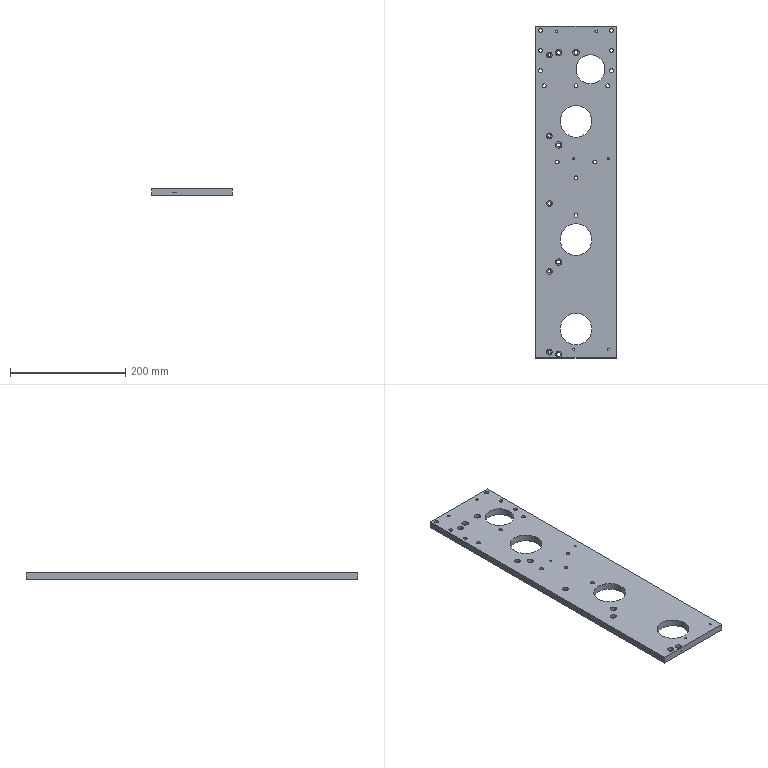Part | NX | 1 solid | 91 faces | box 140 x 575 x 12 mm | volume 838700 mm3 | cylinder 59 | plane 29 | cone 3 | commonest cylinder face diameters 11 x18 6.6 x16 5.5 x5 10 x5 3.3 x4 3 x3